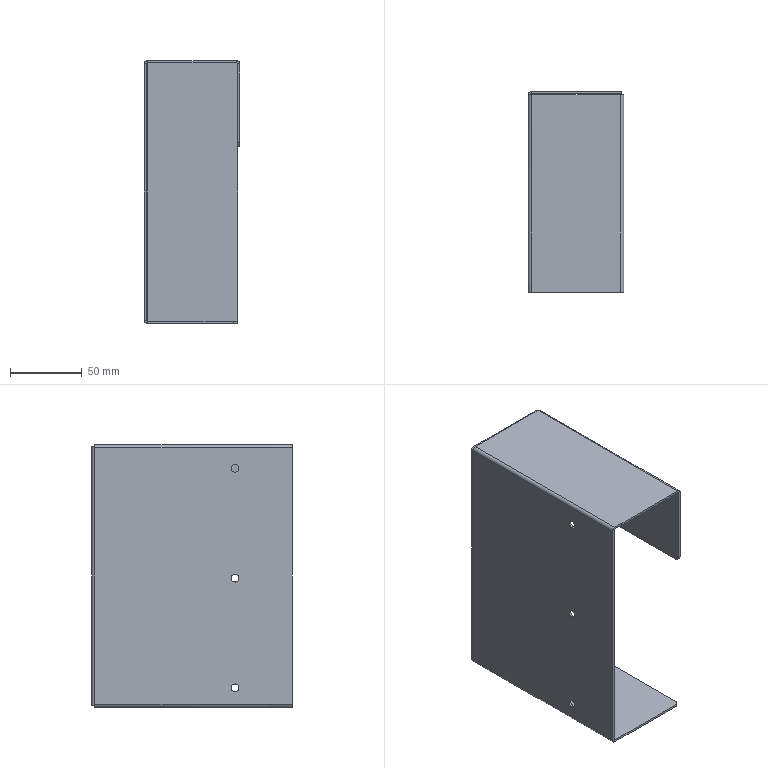Part | SolidWorks | features EdgeFlange 2, Fillet 1, FlatPattern 1, HoleWzd 1, SMBaseFlange 1, SheetMetal 1 | 1 solid | 48 faces | box 66.5 x 140 x 183 mm | volume 93527 mm3 | plane 32 | cylinder 16 | commonest cylinder face diameters 5.5 x6 1.473 x4 4.473 x4 6 x2
STEP:
#1=CARTESIAN_POINT('',(1.5,40.,9.25));
#2=VERTEX_POINT('',#1);
#3=CARTESIAN_POINT('',(1.5,40.,14.75));
#4=VERTEX_POINT('',#3);
#5=CARTESIAN_POINT('',(1.5,40.,12.));
#6=DIRECTION('',(-1.,0.,0.));
#7=DIRECTION('',(0.,0.,1.));
#8=AXIS2_PLACEMENT_3D('',#5,#6,#7);
#9=CIRCLE('',#8,2.75);
#10=EDGE_CURVE('',#2,#4,#9,.T.);
#11=ORIENTED_EDGE('',*,*,#10,.F.);
#12=CARTESIAN_POINT('',(0.,40.,9.25));
#13=VERTEX_POINT('',#12);
#14=CARTESIAN_POINT('',(0.,40.,9.25));
#15=DIRECTION('',(-1.,0.,0.));
#16=VECTOR('',#15,1000.);
#17=LINE('',#14,#16);
#18=EDGE_CURVE('',#2,#13,#17,.T.);
#19=ORIENTED_EDGE('',*,*,#18,.T.);
#20=CARTESIAN_POINT('',(0.,40.,14.75));
#21=VERTEX_POINT('',#20);
#22=CARTESIAN_POINT('',(0.,40.,12.));
#23=DIRECTION('',(-1.,0.,0.));
#24=DIRECTION('',(0.,0.,1.));
#25=AXIS2_PLACEMENT_3D('',#22,#23,#24);
#26=CIRCLE('',#25,2.75);
#27=EDGE_CURVE('',#13,#21,#26,.T.);
#28=ORIENTED_EDGE('',*,*,#27,.T.);
#29=CARTESIAN_POINT('',(0.,40.,14.75));
#30=DIRECTION('',(-1.,0.,0.));
#31=VECTOR('',#30,1000.);
#32=LINE('',#29,#31);
#33=EDGE_CURVE('',#4,#21,#32,.T.);
#34=ORIENTED_EDGE('',*,*,#33,.F.);
#35=EDGE_LOOP('',(#11,#19,#28,#34));
#36=FACE_OUTER_BOUND('',#35,.T.);
#37=CARTESIAN_POINT('',(0.,40.,12.));
#38=DIRECTION('',(-1.,0.,0.));
#39=DIRECTION('',(0.,0.,1.));
#40=AXIS2_PLACEMENT_3D('',#37,#38,#39);
#41=CYLINDRICAL_SURFACE('',#40,2.75);
#42=ADVANCED_FACE('',(#36),#41,.F.);
#43=CARTESIAN_POINT('',(1.5,40.,85.75));
#44=VERTEX_POINT('',#43);
#45=CARTESIAN_POINT('',(1.5,40.,91.25));
#46=VERTEX_POINT('',#45);
#47=CARTESIAN_POINT('',(1.5,40.,88.5));
#48=DIRECTION('',(-1.,0.,0.));
#49=DIRECTION('',(0.,0.,1.));
#50=AXIS2_PLACEMENT_3D('',#47,#48,#49);
#51=CIRCLE('',#50,2.75);
#52=EDGE_CURVE('',#44,#46,#51,.T.);
#53=ORIENTED_EDGE('',*,*,#52,.F.);
#54=CARTESIAN_POINT('',(0.,40.,85.75));
#55=VERTEX_POINT('',#54);
#56=CARTESIAN_POINT('',(0.,40.,85.75));
#57=DIRECTION('',(-1.,0.,0.));
#58=VECTOR('',#57,1000.);
#59=LINE('',#56,#58);
#60=EDGE_CURVE('',#44,#55,#59,.T.);
#61=ORIENTED_EDGE('',*,*,#60,.T.);
#62=CARTESIAN_POINT('',(0.,40.,91.25));
#63=VERTEX_POINT('',#62);
#64=CARTESIAN_POINT('',(0.,40.,88.5));
#65=DIRECTION('',(-1.,0.,0.));
#66=DIRECTION('',(0.,0.,1.));
#67=AXIS2_PLACEMENT_3D('',#64,#65,#66);
#68=CIRCLE('',#67,2.75);
#69=EDGE_CURVE('',#55,#63,#68,.T.);
#70=ORIENTED_EDGE('',*,*,#69,.T.);
#71=CARTESIAN_POINT('',(0.,40.,91.25));
#72=DIRECTION('',(-1.,0.,0.));
#73=VECTOR('',#72,1000.);
#74=LINE('',#71,#73);
#75=EDGE_CURVE('',#46,#63,#74,.T.);
#76=ORIENTED_EDGE('',*,*,#75,.F.);
#77=EDGE_LOOP('',(#53,#61,#70,#76));
#78=FACE_OUTER_BOUND('',#77,.T.);
#79=CARTESIAN_POINT('',(0.,40.,88.5));
#80=DIRECTION('',(-1.,0.,0.));
#81=DIRECTION('',(0.,0.,1.));
#82=AXIS2_PLACEMENT_3D('',#79,#80,#81);
#83=CYLINDRICAL_SURFACE('',#82,2.75);
#84=ADVANCED_FACE('',(#78),#83,.F.);
#85=CARTESIAN_POINT('',(1.5,40.,162.25));
#86=VERTEX_POINT('',#85);
#87=CARTESIAN_POINT('',(1.5,40.,167.75));
#88=VERTEX_POINT('',#87);
#89=CARTESIAN_POINT('',(1.5,40.,165.));
#90=DIRECTION('',(-1.,0.,0.));
#91=DIRECTION('',(0.,0.,1.));
#92=AXIS2_PLACEMENT_3D('',#89,#90,#91);
#93=CIRCLE('',#92,2.75);
#94=EDGE_CURVE('',#86,#88,#93,.T.);
#95=ORIENTED_EDGE('',*,*,#94,.F.);
#96=CARTESIAN_POINT('',(0.,40.,162.25));
#97=VERTEX_POINT('',#96);
#98=CARTESIAN_POINT('',(0.,40.,162.25));
#99=DIRECTION('',(-1.,0.,0.));
#100=VECTOR('',#99,1000.);
#101=LINE('',#98,#100);
#102=EDGE_CURVE('',#86,#97,#101,.T.);
#103=ORIENTED_EDGE('',*,*,#102,.T.);
#104=CARTESIAN_POINT('',(0.,40.,167.75));
#105=VERTEX_POINT('',#104);
#106=CARTESIAN_POINT('',(0.,40.,165.));
#107=DIRECTION('',(-1.,0.,0.));
#108=DIRECTION('',(0.,0.,1.));
#109=AXIS2_PLACEMENT_3D('',#106,#107,#108);
#110=CIRCLE('',#109,2.75);
#111=EDGE_CURVE('',#97,#105,#110,.T.);
#112=ORIENTED_EDGE('',*,*,#111,.T.);
#113=CARTESIAN_POINT('',(0.,40.,167.75));
#114=DIRECTION('',(-1.,0.,0.));
#115=VECTOR('',#114,1000.);
#116=LINE('',#113,#115);
#117=EDGE_CURVE('',#88,#105,#116,.T.);
#118=ORIENTED_EDGE('',*,*,#117,.F.);
#119=EDGE_LOOP('',(#95,#103,#112,#118));
#120=FACE_OUTER_BOUND('',#119,.T.);
#121=CARTESIAN_POINT('',(0.,40.,165.));
#122=DIRECTION('',(-1.,0.,0.));
#123=DIRECTION('',(0.,0.,1.));
#124=AXIS2_PLACEMENT_3D('',#121,#122,#123);
#125=CYLINDRICAL_SURFACE('',#124,2.75);
#126=ADVANCED_FACE('',(#120),#125,.F.);
#127=CARTESIAN_POINT('',(64.263,0.,180.));
#128=VERTEX_POINT('',#127);
#129=CARTESIAN_POINT('',(64.263,0.,181.5));
#130=VERTEX_POINT('',#129);
#131=CARTESIAN_POINT('',(64.263,0.,180.));
#132=DIRECTION('',(0.,0.,1.));
#133=VECTOR('',#132,1000.);
#134=LINE('',#131,#133);
#135=EDGE_CURVE('',#128,#130,#134,.T.);
#136=ORIENTED_EDGE('',*,*,#135,.T.);
#137=CARTESIAN_POINT('',(2.237,0.,181.5));
#138=VERTEX_POINT('',#137);
#139=CARTESIAN_POINT('',(65.,0.,181.5));
#140=DIRECTION('',(1.,0.,0.));
#141=VECTOR('',#140,1000.);
#142=LINE('',#139,#141);
#143=EDGE_CURVE('',#138,#130,#142,.T.);
#144=ORIENTED_EDGE('',*,*,#143,.F.);
#145=CARTESIAN_POINT('',(2.237,0.,180.));
#146=VERTEX_POINT('',#145);
#147=CARTESIAN_POINT('',(2.237,0.,180.));
#148=DIRECTION('',(0.,0.,1.));
#149=VECTOR('',#148,1000.);
#150=LINE('',#147,#149);
#151=EDGE_CURVE('',#146,#138,#150,.T.);
#152=ORIENTED_EDGE('',*,*,#151,.F.);
#153=CARTESIAN_POINT('',(65.,0.,180.));
#154=DIRECTION('',(1.,0.,0.));
#155=VECTOR('',#154,1000.);
#156=LINE('',#153,#155);
#157=EDGE_CURVE('',#146,#128,#156,.T.);
#158=ORIENTED_EDGE('',*,*,#157,.T.);
#159=EDGE_LOOP('',(#136,#144,#152,#158));
#160=FACE_OUTER_BOUND('',#159,.T.);
#161=CARTESIAN_POINT('',(65.,0.,181.5));
#162=DIRECTION('',(0.,1.,0.));
#163=DIRECTION('',(0.,0.,1.));
#164=AXIS2_PLACEMENT_3D('',#161,#162,#163);
#165=PLANE('',#164);
#166=ADVANCED_FACE('',(#160),#165,.F.);
#167=CARTESIAN_POINT('',(64.263,137.763,180.));
#168=VERTEX_POINT('',#167);
#169=CARTESIAN_POINT('',(64.263,137.763,181.5));
#170=VERTEX_POINT('',#169);
#171=CARTESIAN_POINT('',(64.263,137.763,180.));
#172=DIRECTION('',(0.,0.,1.));
#173=VECTOR('',#172,1000.);
#174=LINE('',#171,#173);
#175=EDGE_CURVE('',#168,#170,#174,.T.);
#176=ORIENTED_EDGE('',*,*,#175,.F.);
#177=CARTESIAN_POINT('',(2.237,137.763,180.));
#178=VERTEX_POINT('',#177);
#179=CARTESIAN_POINT('',(1.5,137.763,180.));
#180=DIRECTION('',(-1.,0.,0.));
#181=VECTOR('',#180,1000.);
#182=LINE('',#179,#181);
#183=EDGE_CURVE('',#168,#178,#182,.T.);
#184=ORIENTED_EDGE('',*,*,#183,.T.);
#185=CARTESIAN_POINT('',(2.237,137.763,181.5));
#186=VERTEX_POINT('',#185);
#187=CARTESIAN_POINT('',(2.237,137.763,180.));
#188=DIRECTION('',(0.,0.,1.));
#189=VECTOR('',#188,1000.);
#190=LINE('',#187,#189);
#191=EDGE_CURVE('',#178,#186,#190,.T.);
#192=ORIENTED_EDGE('',*,*,#191,.T.);
#193=CARTESIAN_POINT('',(1.5,137.763,181.5));
#194=DIRECTION('',(-1.,0.,0.));
#195=VECTOR('',#194,1000.);
#196=LINE('',#193,#195);
#197=EDGE_CURVE('',#170,#186,#196,.T.);
#198=ORIENTED_EDGE('',*,*,#197,.F.);
#199=EDGE_LOOP('',(#176,#184,#192,#198));
#200=FACE_OUTER_BOUND('',#199,.T.);
#201=CARTESIAN_POINT('',(1.5,137.763,181.5));
#202=DIRECTION('',(0.,-1.,0.));
#203=DIRECTION('',(0.,0.,-1.));
#204=AXIS2_PLACEMENT_3D('',#201,#202,#203);
#205=PLANE('',#204);
#206=ADVANCED_FACE('',(#200),#205,.F.);
#207=CARTESIAN_POINT('',(64.263,0.,181.5));
#208=DIRECTION('',(0.,1.,0.));
#209=VECTOR('',#208,1000.);
#210=LINE('',#207,#209);
#211=EDGE_CURVE('',#130,#170,#210,.T.);
#212=ORIENTED_EDGE('',*,*,#211,.T.);
#213=ORIENTED_EDGE('',*,*,#197,.T.);
#214=CARTESIAN_POINT('',(2.237,0.,181.5));
#215=DIRECTION('',(0.,1.,0.));
#216=VECTOR('',#215,1000.);
#217=LINE('',#214,#216);
#218=EDGE_CURVE('',#138,#186,#217,.T.);
#219=ORIENTED_EDGE('',*,*,#218,.F.);
#220=ORIENTED_EDGE('',*,*,#143,.T.);
#221=EDGE_LOOP('',(#212,#213,#219,#220));
#222=FACE_OUTER_BOUND('',#221,.T.);
#223=CARTESIAN_POINT('',(0.,0.,181.5));
#224=DIRECTION('',(0.,0.,-1.));
#225=DIRECTION('',(-1.,0.,0.));
#226=AXIS2_PLACEMENT_3D('',#223,#224,#225);
#227=PLANE('',#226);
#228=ADVANCED_FACE('',(#222),#227,.F.);
#229=ORIENTED_EDGE('',*,*,#183,.F.);
#230=CARTESIAN_POINT('',(64.263,0.,180.));
#231=DIRECTION('',(0.,1.,0.));
#232=VECTOR('',#231,1000.);
#233=LINE('',#230,#232);
#234=EDGE_CURVE('',#128,#168,#233,.T.);
#235=ORIENTED_EDGE('',*,*,#234,.F.);
#236=ORIENTED_EDGE('',*,*,#157,.F.);
#237=CARTESIAN_POINT('',(2.237,137.763,180.));
#238=DIRECTION('',(0.,-1.,0.));
#239=VECTOR('',#238,1000.);
#240=LINE('',#237,#239);
#241=EDGE_CURVE('',#178,#146,#240,.T.);
#242=ORIENTED_EDGE('',*,*,#241,.F.);
#243=EDGE_LOOP('',(#229,#235,#236,#242));
#244=FACE_OUTER_BOUND('',#243,.T.);
#245=CARTESIAN_POINT('',(0.,0.,180.));
#246=DIRECTION('',(0.,0.,-1.));
#247=DIRECTION('',(-1.,0.,0.));
#248=AXIS2_PLACEMENT_3D('',#245,#246,#247);
#249=PLANE('',#248);
#250=ADVANCED_FACE('',(#244),#249,.T.);
#251=CARTESIAN_POINT('',(0.,137.763,180.));
#252=VERTEX_POINT('',#251);
#253=CARTESIAN_POINT('',(0.,137.763,179.263));
#254=VERTEX_POINT('',#253);
#255=CARTESIAN_POINT('',(0.,137.763,180.));
#256=DIRECTION('',(0.,0.,-1.));
#257=VECTOR('',#256,1000.);
#258=LINE('',#255,#257);
#259=EDGE_CURVE('',#252,#254,#258,.T.);
#260=ORIENTED_EDGE('',*,*,#259,.T.);
#261=CARTESIAN_POINT('',(0.1248,137.763,180.));
#262=VERTEX_POINT('',#261);
#263=CARTESIAN_POINT('',(2.237,137.763,179.263));
#264=DIRECTION('',(0.,1.,0.));
#265=DIRECTION('',(0.,0.,-1.));
#266=AXIS2_PLACEMENT_3D('',#263,#264,#265);
#267=CIRCLE('',#266,2.237);
#268=EDGE_CURVE('',#254,#262,#267,.T.);
#269=ORIENTED_EDGE('',*,*,#268,.T.);
#270=CARTESIAN_POINT('',(1.5,137.763,180.));
#271=DIRECTION('',(-1.,0.,0.));
#272=VECTOR('',#271,1000.);
#273=LINE('',#270,#272);
#274=EDGE_CURVE('',#262,#252,#273,.T.);
#275=ORIENTED_EDGE('',*,*,#274,.T.);
#276=EDGE_LOOP('',(#260,#269,#275));
#277=FACE_OUTER_BOUND('',#276,.T.);
#278=CARTESIAN_POINT('',(1.5,137.763,179.263));
#279=DIRECTION('',(0.,-1.,0.));
#280=DIRECTION('',(0.,0.,-1.));
#281=AXIS2_PLACEMENT_3D('',#278,#279,#280);
#282=PLANE('',#281);
#283=ADVANCED_FACE('',(#277),#282,.T.);
#284=CARTESIAN_POINT('',(0.,137.763,0.));
#285=VERTEX_POINT('',#284);
#286=CARTESIAN_POINT('',(0.1248,137.763,0.));
#287=VERTEX_POINT('',#286);
#288=CARTESIAN_POINT('',(0.,137.763,0.));
#289=DIRECTION('',(1.,0.,0.));
#290=VECTOR('',#289,1000.);
#291=LINE('',#288,#290);
#292=EDGE_CURVE('',#285,#287,#291,.T.);
#293=ORIENTED_EDGE('',*,*,#292,.T.);
#294=CARTESIAN_POINT('',(0.,137.763,0.7366));
#295=VERTEX_POINT('',#294);
#296=CARTESIAN_POINT('',(2.237,137.763,0.7366));
#297=DIRECTION('',(0.,1.,0.));
#298=DIRECTION('',(0.,0.,1.));
#299=AXIS2_PLACEMENT_3D('',#296,#297,#298);
#300=CIRCLE('',#299,2.237);
#301=EDGE_CURVE('',#287,#295,#300,.T.);
#302=ORIENTED_EDGE('',*,*,#301,.T.);
#303=CARTESIAN_POINT('',(0.,137.763,180.));
#304=DIRECTION('',(0.,0.,1.));
#305=VECTOR('',#304,1000.);
#306=LINE('',#303,#305);
#307=EDGE_CURVE('',#285,#295,#306,.T.);
#308=ORIENTED_EDGE('',*,*,#307,.F.);
#309=EDGE_LOOP('',(#293,#302,#308));
#310=FACE_OUTER_BOUND('',#309,.T.);
#311=CARTESIAN_POINT('',(1.5,137.763,0.));
#312=DIRECTION('',(0.,-1.,0.));
#313=DIRECTION('',(0.,0.,-1.));
#314=AXIS2_PLACEMENT_3D('',#311,#312,#313);
#315=PLANE('',#314);
#316=ADVANCED_FACE('',(#310),#315,.T.);
#317=CARTESIAN_POINT('',(0.,40.,12.));
#318=DIRECTION('',(-1.,0.,0.));
#319=DIRECTION('',(0.,0.,1.));
#320=AXIS2_PLACEMENT_3D('',#317,#318,#319);
#321=CIRCLE('',#320,2.75);
#322=EDGE_CURVE('',#21,#13,#321,.T.);
#323=ORIENTED_EDGE('',*,*,#322,.F.);
#324=ORIENTED_EDGE('',*,*,#27,.F.);
#325=EDGE_LOOP('',(#323,#324));
#326=FACE_BOUND('',#325,.T.);
#327=CARTESIAN_POINT('',(0.,40.,88.5));
#328=DIRECTION('',(-1.,0.,0.));
#329=DIRECTION('',(0.,0.,1.));
#330=AXIS2_PLACEMENT_3D('',#327,#328,#329);
#331=CIRCLE('',#330,2.75);
#332=EDGE_CURVE('',#63,#55,#331,.T.);
#333=ORIENTED_EDGE('',*,*,#332,.F.);
#334=ORIENTED_EDGE('',*,*,#69,.F.);
#335=EDGE_LOOP('',(#333,#334));
#336=FACE_BOUND('',#335,.T.);
#337=CARTESIAN_POINT('',(0.,40.,165.));
#338=DIRECTION('',(-1.,0.,0.));
#339=DIRECTION('',(0.,0.,1.));
#340=AXIS2_PLACEMENT_3D('',#337,#338,#339);
#341=CIRCLE('',#340,2.75);
#342=EDGE_CURVE('',#105,#97,#341,.T.);
#343=ORIENTED_EDGE('',*,*,#342,.F.);
#344=ORIENTED_EDGE('',*,*,#111,.F.);
#345=EDGE_LOOP('',(#343,#344));
#346=FACE_BOUND('',#345,.T.);
#347=CARTESIAN_POINT('',(0.,0.,179.263));
#348=VERTEX_POINT('',#347);
#349=CARTESIAN_POINT('',(0.,0.,0.7366));
#350=VERTEX_POINT('',#349);
#351=CARTESIAN_POINT('',(0.,0.,180.));
#352=DIRECTION('',(0.,0.,-1.));
#353=VECTOR('',#352,1000.);
#354=LINE('',#351,#353);
#355=EDGE_CURVE('',#348,#350,#354,.T.);
#356=ORIENTED_EDGE('',*,*,#355,.F.);
#357=CARTESIAN_POINT('',(0.,0.,179.263));
#358=DIRECTION('',(0.,1.,0.));
#359=VECTOR('',#358,1000.);
#360=LINE('',#357,#359);
#361=EDGE_CURVE('',#348,#254,#360,.T.);
#362=ORIENTED_EDGE('',*,*,#361,.T.);
#363=CARTESIAN_POINT('',(0.,137.763,180.));
#364=DIRECTION('',(0.,0.,-1.));
#365=VECTOR('',#364,1000.);
#366=LINE('',#363,#365);
#367=EDGE_CURVE('',#254,#295,#366,.T.);
#368=ORIENTED_EDGE('',*,*,#367,.T.);
#369=CARTESIAN_POINT('',(0.,137.763,0.7366));
#370=DIRECTION('',(0.,-1.,0.));
#371=VECTOR('',#370,1000.);
#372=LINE('',#369,#371);
#373=EDGE_CURVE('',#295,#350,#372,.T.);
#374=ORIENTED_EDGE('',*,*,#373,.T.);
#375=EDGE_LOOP('',(#356,#362,#368,#374));
#376=FACE_OUTER_BOUND('',#375,.T.);
#377=CARTESIAN_POINT('',(0.,0.,180.));
#378=DIRECTION('',(-1.,0.,0.));
#379=DIRECTION('',(0.,0.,1.));
#380=AXIS2_PLACEMENT_3D('',#377,#378,#379);
#381=PLANE('',#380);
#382=ADVANCED_FACE('',(#326,#336,#346,#376),#381,.T.);
#383=CARTESIAN_POINT('',(1.5,40.,12.));
#384=DIRECTION('',(-1.,0.,0.));
#385=DIRECTION('',(0.,0.,1.));
#386=AXIS2_PLACEMENT_3D('',#383,#384,#385);
#387=CIRCLE('',#386,2.75);
#388=EDGE_CURVE('',#4,#2,#387,.T.);
#389=ORIENTED_EDGE('',*,*,#388,.T.);
#390=ORIENTED_EDGE('',*,*,#10,.T.);
#391=EDGE_LOOP('',(#389,#390));
#392=FACE_BOUND('',#391,.T.);
#393=CARTESIAN_POINT('',(1.5,40.,88.5));
#394=DIRECTION('',(-1.,0.,0.));
#395=DIRECTION('',(0.,0.,1.));
#396=AXIS2_PLACEMENT_3D('',#393,#394,#395);
#397=CIRCLE('',#396,2.75);
#398=EDGE_CURVE('',#46,#44,#397,.T.);
#399=ORIENTED_EDGE('',*,*,#398,.T.);
#400=ORIENTED_EDGE('',*,*,#52,.T.);
#401=EDGE_LOOP('',(#399,#400));
#402=FACE_BOUND('',#401,.T.);
#403=CARTESIAN_POINT('',(1.5,40.,165.));
#404=DIRECTION('',(-1.,0.,0.));
#405=DIRECTION('',(0.,0.,1.));
#406=AXIS2_PLACEMENT_3D('',#403,#404,#405);
#407=CIRCLE('',#406,2.75);
#408=EDGE_CURVE('',#88,#86,#407,.T.);
#409=ORIENTED_EDGE('',*,*,#408,.T.);
#410=ORIENTED_EDGE('',*,*,#94,.T.);
#411=EDGE_LOOP('',(#409,#410));
#412=FACE_BOUND('',#411,.T.);
#413=CARTESIAN_POINT('',(1.5,0.,179.263));
#414=VERTEX_POINT('',#413);
#415=CARTESIAN_POINT('',(1.5,137.763,179.263));
#416=VERTEX_POINT('',#415);
#417=CARTESIAN_POINT('',(1.5,0.,179.263));
#418=DIRECTION('',(0.,1.,0.));
#419=VECTOR('',#418,1000.);
#420=LINE('',#417,#419);
#421=EDGE_CURVE('',#414,#416,#420,.T.);
#422=ORIENTED_EDGE('',*,*,#421,.F.);
#423=CARTESIAN_POINT('',(1.5,0.,0.7366));
#424=VERTEX_POINT('',#423);
#425=CARTESIAN_POINT('',(1.5,0.,180.));
#426=DIRECTION('',(0.,0.,-1.));
#427=VECTOR('',#426,1000.);
#428=LINE('',#425,#427);
#429=EDGE_CURVE('',#414,#424,#428,.T.);
#430=ORIENTED_EDGE('',*,*,#429,.T.);
#431=CARTESIAN_POINT('',(1.5,137.763,0.7366));
#432=VERTEX_POINT('',#431);
#433=CARTESIAN_POINT('',(1.5,137.763,0.7366));
#434=DIRECTION('',(0.,-1.,0.));
#435=VECTOR('',#434,1000.);
#436=LINE('',#433,#435);
#437=EDGE_CURVE('',#432,#424,#436,.T.);
#438=ORIENTED_EDGE('',*,*,#437,.F.);
#439=CARTESIAN_POINT('',(1.5,137.763,180.));
#440=DIRECTION('',(0.,0.,-1.));
#441=VECTOR('',#440,1000.);
#442=LINE('',#439,#441);
#443=EDGE_CURVE('',#416,#432,#442,.T.);
#444=ORIENTED_EDGE('',*,*,#443,.F.);
#445=EDGE_LOOP('',(#422,#430,#438,#444));
#446=FACE_OUTER_BOUND('',#445,.T.);
#447=CARTESIAN_POINT('',(1.5,0.,180.));
#448=DIRECTION('',(-1.,0.,0.));
#449=DIRECTION('',(0.,0.,1.));
#450=AXIS2_PLACEMENT_3D('',#447,#448,#449);
#451=PLANE('',#450);
#452=ADVANCED_FACE('',(#392,#402,#412,#446),#451,.F.);
#453=ORIENTED_EDGE('',*,*,#429,.F.);
#454=CARTESIAN_POINT('',(1.5,0.,179.263));
#455=DIRECTION('',(-1.,0.,0.));
#456=VECTOR('',#455,1000.);
#457=LINE('',#454,#456);
#458=EDGE_CURVE('',#414,#348,#457,.T.);
#459=ORIENTED_EDGE('',*,*,#458,.T.);
#460=ORIENTED_EDGE('',*,*,#355,.T.);
#461=CARTESIAN_POINT('',(1.5,0.,0.7366));
#462=DIRECTION('',(-1.,0.,0.));
#463=VECTOR('',#462,1000.);
#464=LINE('',#461,#463);
#465=EDGE_CURVE('',#424,#350,#464,.T.);
#466=ORIENTED_EDGE('',*,*,#465,.F.);
#467=EDGE_LOOP('',(#453,#459,#460,#466));
#468=FACE_OUTER_BOUND('',#467,.T.);
#469=CARTESIAN_POINT('',(1.5,0.,180.));
#470=DIRECTION('',(0.,-1.,0.));
#471=DIRECTION('',(0.,0.,-1.));
#472=AXIS2_PLACEMENT_3D('',#469,#470,#471);
#473=PLANE('',#472);
#474=ADVANCED_FACE('',(#468),#473,.T.);
#475=CARTESIAN_POINT('',(2.237,140.,180.));
#476=VERTEX_POINT('',#475);
#477=CARTESIAN_POINT('',(2.237,138.5,180.));
#478=VERTEX_POINT('',#477);
#479=CARTESIAN_POINT('',(2.237,140.,180.));
#480=DIRECTION('',(0.,-1.,0.));
#481=VECTOR('',#480,1000.);
#482=LINE('',#479,#481);
#483=EDGE_CURVE('',#476,#478,#482,.T.);
#484=ORIENTED_EDGE('',*,*,#483,.F.);
#485=CARTESIAN_POINT('',(2.237,137.763,180.));
#486=DIRECTION('',(0.,0.,-1.));
#487=DIRECTION('',(1.,0.,0.));
#488=AXIS2_PLACEMENT_3D('',#485,#486,#487);
#489=CIRCLE('',#488,2.237);
#490=EDGE_CURVE('',#252,#476,#489,.T.);
#491=ORIENTED_EDGE('',*,*,#490,.F.);
#492=ORIENTED_EDGE('',*,*,#274,.F.);
#493=CARTESIAN_POINT('',(1.5,137.763,180.));
#494=VERTEX_POINT('',#493);
#495=CARTESIAN_POINT('',(1.5,137.763,180.));
#496=DIRECTION('',(-1.,0.,0.));
#497=VECTOR('',#496,1000.);
#498=LINE('',#495,#497);
#499=EDGE_CURVE('',#494,#262,#498,.T.);
#500=ORIENTED_EDGE('',*,*,#499,.F.);
#501=CARTESIAN_POINT('',(2.237,137.763,180.));
#502=DIRECTION('',(0.,0.,-1.));
#503=DIRECTION('',(1.,0.,0.));
#504=AXIS2_PLACEMENT_3D('',#501,#502,#503);
#505=CIRCLE('',#504,0.7366);
#506=EDGE_CURVE('',#494,#478,#505,.T.);
#507=ORIENTED_EDGE('',*,*,#506,.T.);
#508=EDGE_LOOP('',(#484,#491,#492,#500,#507));
#509=FACE_OUTER_BOUND('',#508,.T.);
#510=CARTESIAN_POINT('',(2.237,140.,180.));
#511=DIRECTION('',(0.,0.,1.));
#512=DIRECTION('',(1.,0.,0.));
#513=AXIS2_PLACEMENT_3D('',#510,#511,#512);
#514=PLANE('',#513);
#515=ADVANCED_FACE('',(#509),#514,.T.);
#516=CARTESIAN_POINT('',(65.,140.,180.));
#517=VERTEX_POINT('',#516);
#518=CARTESIAN_POINT('',(0.,140.,180.));
#519=DIRECTION('',(1.,0.,0.));
#520=VECTOR('',#519,1000.);
#521=LINE('',#518,#520);
#522=EDGE_CURVE('',#476,#517,#521,.T.);
#523=ORIENTED_EDGE('',*,*,#522,.F.);
#524=ORIENTED_EDGE('',*,*,#483,.T.);
#525=CARTESIAN_POINT('',(65.,138.5,180.));
#526=VERTEX_POINT('',#525);
#527=CARTESIAN_POINT('',(0.,138.5,180.));
#528=DIRECTION('',(1.,0.,0.));
#529=VECTOR('',#528,1000.);
#530=LINE('',#527,#529);
#531=EDGE_CURVE('',#478,#526,#530,.T.);
#532=ORIENTED_EDGE('',*,*,#531,.T.);
#533=CARTESIAN_POINT('',(65.,140.,180.));
#534=DIRECTION('',(0.,-1.,0.));
#535=VECTOR('',#534,1000.);
#536=LINE('',#533,#535);
#537=EDGE_CURVE('',#517,#526,#536,.T.);
#538=ORIENTED_EDGE('',*,*,#537,.F.);
#539=EDGE_LOOP('',(#523,#524,#532,#538));
#540=FACE_OUTER_BOUND('',#539,.T.);
#541=CARTESIAN_POINT('',(1.5,137.763,180.));
#542=DIRECTION('',(0.,0.,1.));
#543=DIRECTION('',(1.,0.,0.));
#544=AXIS2_PLACEMENT_3D('',#541,#542,#543);
#545=PLANE('',#544);
#546=ADVANCED_FACE('',(#540),#545,.T.);
#547=ORIENTED_EDGE('',*,*,#292,.F.);
#548=CARTESIAN_POINT('',(2.237,140.,0.));
#549=VERTEX_POINT('',#548);
#550=CARTESIAN_POINT('',(2.237,137.763,0.));
#551=DIRECTION('',(0.,0.,-1.));
#552=DIRECTION('',(1.,0.,0.));
#553=AXIS2_PLACEMENT_3D('',#550,#551,#552);
#554=CIRCLE('',#553,2.237);
#555=EDGE_CURVE('',#285,#549,#554,.T.);
#556=ORIENTED_EDGE('',*,*,#555,.T.);
#557=CARTESIAN_POINT('',(2.237,138.5,0.));
#558=VERTEX_POINT('',#557);
#559=CARTESIAN_POINT('',(2.237,138.5,0.));
#560=DIRECTION('',(0.,1.,0.));
#561=VECTOR('',#560,1000.);
#562=LINE('',#559,#561);
#563=EDGE_CURVE('',#558,#549,#562,.T.);
#564=ORIENTED_EDGE('',*,*,#563,.F.);
#565=CARTESIAN_POINT('',(1.5,137.763,0.));
#566=VERTEX_POINT('',#565);
#567=CARTESIAN_POINT('',(2.237,137.763,0.));
#568=DIRECTION('',(0.,0.,-1.));
#569=DIRECTION('',(1.,0.,0.));
#570=AXIS2_PLACEMENT_3D('',#567,#568,#569);
#571=CIRCLE('',#570,0.7366);
#572=EDGE_CURVE('',#566,#558,#571,.T.);
#573=ORIENTED_EDGE('',*,*,#572,.F.);
#574=CARTESIAN_POINT('',(0.,137.763,0.));
#575=DIRECTION('',(1.,0.,0.));
#576=VECTOR('',#575,1000.);
#577=LINE('',#574,#576);
#578=EDGE_CURVE('',#287,#566,#577,.T.);
#579=ORIENTED_EDGE('',*,*,#578,.F.);
#580=EDGE_LOOP('',(#547,#556,#564,#573,#579));
#581=FACE_OUTER_BOUND('',#580,.T.);
#582=CARTESIAN_POINT('',(0.,137.763,0.));
#583=DIRECTION('',(0.,0.,-1.));
#584=DIRECTION('',(-1.,0.,0.));
#585=AXIS2_PLACEMENT_3D('',#582,#583,#584);
#586=PLANE('',#585);
#587=ADVANCED_FACE('',(#581),#586,.T.);
#588=CARTESIAN_POINT('',(65.,138.5,0.));
#589=VERTEX_POINT('',#588);
#590=CARTESIAN_POINT('',(0.,138.5,0.));
#591=DIRECTION('',(1.,0.,0.));
#592=VECTOR('',#591,1000.);
#593=LINE('',#590,#592);
#594=EDGE_CURVE('',#558,#589,#593,.T.);
#595=ORIENTED_EDGE('',*,*,#594,.T.);
#596=CARTESIAN_POINT('',(65.,138.5,180.));
#597=DIRECTION('',(0.,0.,-1.));
#598=VECTOR('',#597,1000.);
#599=LINE('',#596,#598);
#600=EDGE_CURVE('',#526,#589,#599,.T.);
#601=ORIENTED_EDGE('',*,*,#600,.F.);
#602=ORIENTED_EDGE('',*,*,#531,.F.);
#603=CARTESIAN_POINT('',(2.237,138.5,180.));
#604=DIRECTION('',(0.,0.,-1.));
#605=VECTOR('',#604,1000.);
#606=LINE('',#603,#605);
#607=EDGE_CURVE('',#478,#558,#606,.T.);
#608=ORIENTED_EDGE('',*,*,#607,.T.);
#609=EDGE_LOOP('',(#595,#601,#602,#608));
#610=FACE_OUTER_BOUND('',#609,.T.);
#611=CARTESIAN_POINT('',(0.,138.5,180.));
#612=DIRECTION('',(0.,1.,0.));
#613=DIRECTION('',(0.,0.,1.));
#614=AXIS2_PLACEMENT_3D('',#611,#612,#613);
#615=PLANE('',#614);
#616=ADVANCED_FACE('',(#610),#615,.F.);
#617=CARTESIAN_POINT('',(65.,140.,0.));
#618=VERTEX_POINT('',#617);
#619=CARTESIAN_POINT('',(65.,140.,0.));
#620=DIRECTION('',(0.,-1.,0.));
#621=VECTOR('',#620,1000.);
#622=LINE('',#619,#621);
#623=EDGE_CURVE('',#618,#589,#622,.T.);
#624=ORIENTED_EDGE('',*,*,#623,.F.);
#625=CARTESIAN_POINT('',(65.,140.,180.));
#626=DIRECTION('',(0.,0.,-1.));
#627=VECTOR('',#626,1000.);
#628=LINE('',#625,#627);
#629=EDGE_CURVE('',#517,#618,#628,.T.);
#630=ORIENTED_EDGE('',*,*,#629,.F.);
#631=ORIENTED_EDGE('',*,*,#537,.T.);
#632=ORIENTED_EDGE('',*,*,#600,.T.);
#633=EDGE_LOOP('',(#624,#630,#631,#632));
#634=FACE_OUTER_BOUND('',#633,.T.);
#635=CARTESIAN_POINT('',(65.,140.,180.));
#636=DIRECTION('',(1.,0.,0.));
#637=DIRECTION('',(0.,0.,-1.));
#638=AXIS2_PLACEMENT_3D('',#635,#636,#637);
#639=PLANE('',#638);
#640=ADVANCED_FACE('',(#634),#639,.T.);
#641=CARTESIAN_POINT('',(0.,140.,0.));
#642=DIRECTION('',(1.,0.,0.));
#643=VECTOR('',#642,1000.);
#644=LINE('',#641,#643);
#645=EDGE_CURVE('',#549,#618,#644,.T.);
#646=ORIENTED_EDGE('',*,*,#645,.F.);
#647=CARTESIAN_POINT('',(2.237,140.,180.));
#648=DIRECTION('',(0.,0.,-1.));
#649=VECTOR('',#648,1000.);
#650=LINE('',#647,#649);
#651=EDGE_CURVE('',#476,#549,#650,.T.);
#652=ORIENTED_EDGE('',*,*,#651,.F.);
#653=ORIENTED_EDGE('',*,*,#522,.T.);
#654=ORIENTED_EDGE('',*,*,#629,.T.);
#655=EDGE_LOOP('',(#646,#652,#653,#654));
#656=FACE_OUTER_BOUND('',#655,.T.);
#657=CARTESIAN_POINT('',(0.,140.,180.));
#658=DIRECTION('',(0.,1.,0.));
#659=DIRECTION('',(0.,0.,1.));
#660=AXIS2_PLACEMENT_3D('',#657,#658,#659);
#661=PLANE('',#660);
#662=ADVANCED_FACE('',(#656),#661,.T.);
#663=ORIENTED_EDGE('',*,*,#555,.F.);
#664=ORIENTED_EDGE('',*,*,#307,.T.);
#665=ORIENTED_EDGE('',*,*,#367,.F.);
#666=ORIENTED_EDGE('',*,*,#259,.F.);
#667=ORIENTED_EDGE('',*,*,#490,.T.);
#668=ORIENTED_EDGE('',*,*,#651,.T.);
#669=EDGE_LOOP('',(#663,#664,#665,#666,#667,#668));
#670=FACE_OUTER_BOUND('',#669,.T.);
#671=CARTESIAN_POINT('',(2.237,137.763,180.));
#672=DIRECTION('',(0.,0.,-1.));
#673=DIRECTION('',(-1.,0.,0.));
#674=AXIS2_PLACEMENT_3D('',#671,#672,#673);
#675=CYLINDRICAL_SURFACE('',#674,2.237);
#676=ADVANCED_FACE('',(#670),#675,.T.);
#677=ORIENTED_EDGE('',*,*,#572,.T.);
#678=ORIENTED_EDGE('',*,*,#607,.F.);
#679=ORIENTED_EDGE('',*,*,#506,.F.);
#680=CARTESIAN_POINT('',(1.5,137.763,180.));
#681=DIRECTION('',(0.,0.,-1.));
#682=VECTOR('',#681,1000.);
#683=LINE('',#680,#682);
#684=EDGE_CURVE('',#494,#416,#683,.T.);
#685=ORIENTED_EDGE('',*,*,#684,.T.);
#686=ORIENTED_EDGE('',*,*,#443,.T.);
#687=CARTESIAN_POINT('',(1.5,137.763,0.));
#688=DIRECTION('',(0.,0.,1.));
#689=VECTOR('',#688,1000.);
#690=LINE('',#687,#689);
#691=EDGE_CURVE('',#566,#432,#690,.T.);
#692=ORIENTED_EDGE('',*,*,#691,.F.);
#693=EDGE_LOOP('',(#677,#678,#679,#685,#686,#692));
#694=FACE_OUTER_BOUND('',#693,.T.);
#695=CARTESIAN_POINT('',(2.237,137.763,180.));
#696=DIRECTION('',(0.,0.,-1.));
#697=DIRECTION('',(-1.,0.,0.));
#698=AXIS2_PLACEMENT_3D('',#695,#696,#697);
#699=CYLINDRICAL_SURFACE('',#698,0.7366);
#700=ADVANCED_FACE('',(#694),#699,.F.);
#701=ORIENTED_EDGE('',*,*,#594,.F.);
#702=ORIENTED_EDGE('',*,*,#563,.T.);
#703=ORIENTED_EDGE('',*,*,#645,.T.);
#704=ORIENTED_EDGE('',*,*,#623,.T.);
#705=EDGE_LOOP('',(#701,#702,#703,#704));
#706=FACE_OUTER_BOUND('',#705,.T.);
#707=CARTESIAN_POINT('',(2.237,137.763,0.));
#708=DIRECTION('',(0.,0.,1.));
#709=DIRECTION('',(1.,0.,0.));
#710=AXIS2_PLACEMENT_3D('',#707,#708,#709);
#711=PLANE('',#710);
#712=ADVANCED_FACE('',(#706),#711,.F.);
#713=ORIENTED_EDGE('',*,*,#102,.F.);
#714=ORIENTED_EDGE('',*,*,#408,.F.);
#715=ORIENTED_EDGE('',*,*,#117,.T.);
#716=ORIENTED_EDGE('',*,*,#342,.T.);
#717=EDGE_LOOP('',(#713,#714,#715,#716));
#718=FACE_OUTER_BOUND('',#717,.T.);
#719=CARTESIAN_POINT('',(0.,40.,165.));
#720=DIRECTION('',(-1.,0.,0.));
#721=DIRECTION('',(0.,0.,1.));
#722=AXIS2_PLACEMENT_3D('',#719,#720,#721);
#723=CYLINDRICAL_SURFACE('',#722,2.75);
#724=ADVANCED_FACE('',(#718),#723,.F.);
#725=ORIENTED_EDGE('',*,*,#60,.F.);
#726=ORIENTED_EDGE('',*,*,#398,.F.);
#727=ORIENTED_EDGE('',*,*,#75,.T.);
#728=ORIENTED_EDGE('',*,*,#332,.T.);
#729=EDGE_LOOP('',(#725,#726,#727,#728));
#730=FACE_OUTER_BOUND('',#729,.T.);
#731=CARTESIAN_POINT('',(0.,40.,88.5));
#732=DIRECTION('',(-1.,0.,0.));
#733=DIRECTION('',(0.,0.,1.));
#734=AXIS2_PLACEMENT_3D('',#731,#732,#733);
#735=CYLINDRICAL_SURFACE('',#734,2.75);
#736=ADVANCED_FACE('',(#730),#735,.F.);
#737=ORIENTED_EDGE('',*,*,#18,.F.);
#738=ORIENTED_EDGE('',*,*,#388,.F.);
#739=ORIENTED_EDGE('',*,*,#33,.T.);
#740=ORIENTED_EDGE('',*,*,#322,.T.);
#741=EDGE_LOOP('',(#737,#738,#739,#740));
#742=FACE_OUTER_BOUND('',#741,.T.);
#743=CARTESIAN_POINT('',(0.,40.,12.));
#744=DIRECTION('',(-1.,0.,0.));
#745=DIRECTION('',(0.,0.,1.));
#746=AXIS2_PLACEMENT_3D('',#743,#744,#745);
#747=CYLINDRICAL_SURFACE('',#746,2.75);
#748=ADVANCED_FACE('',(#742),#747,.F.);
#749=CARTESIAN_POINT('',(2.237,0.,0.));
#750=VERTEX_POINT('',#749);
#751=CARTESIAN_POINT('',(2.237,0.,-1.5));
#752=VERTEX_POINT('',#751);
#753=CARTESIAN_POINT('',(2.237,0.,0.));
#754=DIRECTION('',(0.,0.,-1.));
#755=VECTOR('',#754,1000.);
#756=LINE('',#753,#755);
#757=EDGE_CURVE('',#750,#752,#756,.T.);
#758=ORIENTED_EDGE('',*,*,#757,.F.);
#759=CARTESIAN_POINT('',(2.237,0.,0.7366));
#760=DIRECTION('',(0.,-1.,0.));
#761=DIRECTION('',(0.,0.,1.));
#762=AXIS2_PLACEMENT_3D('',#759,#760,#761);
#763=CIRCLE('',#762,0.7366);
#764=EDGE_CURVE('',#424,#750,#763,.T.);
#765=ORIENTED_EDGE('',*,*,#764,.F.);
#766=ORIENTED_EDGE('',*,*,#465,.T.);
#767=CARTESIAN_POINT('',(2.237,0.,0.7366));
#768=DIRECTION('',(0.,-1.,0.));
#769=DIRECTION('',(0.,0.,1.));
#770=AXIS2_PLACEMENT_3D('',#767,#768,#769);
#771=CIRCLE('',#770,2.237);
#772=EDGE_CURVE('',#350,#752,#771,.T.);
#773=ORIENTED_EDGE('',*,*,#772,.T.);
#774=EDGE_LOOP('',(#758,#765,#766,#773));
#775=FACE_OUTER_BOUND('',#774,.T.);
#776=CARTESIAN_POINT('',(2.237,0.,0.7366));
#777=DIRECTION('',(0.,-1.,0.));
#778=DIRECTION('',(0.,0.,-1.));
#779=AXIS2_PLACEMENT_3D('',#776,#777,#778);
#780=PLANE('',#779);
#781=ADVANCED_FACE('',(#775),#780,.T.);
#782=CARTESIAN_POINT('',(2.237,137.763,-1.5));
#783=VERTEX_POINT('',#782);
#784=CARTESIAN_POINT('',(2.237,137.763,0.7366));
#785=DIRECTION('',(0.,1.,0.));
#786=DIRECTION('',(0.,0.,1.));
#787=AXIS2_PLACEMENT_3D('',#784,#785,#786);
#788=CIRCLE('',#787,2.237);
#789=EDGE_CURVE('',#783,#287,#788,.T.);
#790=ORIENTED_EDGE('',*,*,#789,.T.);
#791=ORIENTED_EDGE('',*,*,#578,.T.);
#792=ORIENTED_EDGE('',*,*,#691,.T.);
#793=CARTESIAN_POINT('',(2.237,137.763,0.));
#794=VERTEX_POINT('',#793);
#795=CARTESIAN_POINT('',(2.237,137.763,0.7366));
#796=DIRECTION('',(0.,1.,0.));
#797=DIRECTION('',(0.,0.,1.));
#798=AXIS2_PLACEMENT_3D('',#795,#796,#797);
#799=CIRCLE('',#798,0.7366);
#800=EDGE_CURVE('',#794,#432,#799,.T.);
#801=ORIENTED_EDGE('',*,*,#800,.F.);
#802=CARTESIAN_POINT('',(2.237,137.763,0.));
#803=DIRECTION('',(0.,0.,-1.));
#804=VECTOR('',#803,1000.);
#805=LINE('',#802,#804);
#806=EDGE_CURVE('',#794,#783,#805,.T.);
#807=ORIENTED_EDGE('',*,*,#806,.T.);
#808=EDGE_LOOP('',(#790,#791,#792,#801,#807));
#809=FACE_OUTER_BOUND('',#808,.T.);
#810=CARTESIAN_POINT('',(2.237,137.763,0.7366));
#811=DIRECTION('',(0.,-1.,0.));
#812=DIRECTION('',(0.,0.,-1.));
#813=AXIS2_PLACEMENT_3D('',#810,#811,#812);
#814=PLANE('',#813);
#815=ADVANCED_FACE('',(#809),#814,.F.);
#816=ORIENTED_EDGE('',*,*,#373,.F.);
#817=ORIENTED_EDGE('',*,*,#301,.F.);
#818=ORIENTED_EDGE('',*,*,#789,.F.);
#819=CARTESIAN_POINT('',(2.237,0.,-1.5));
#820=DIRECTION('',(0.,-1.,0.));
#821=VECTOR('',#820,1000.);
#822=LINE('',#819,#821);
#823=EDGE_CURVE('',#783,#752,#822,.T.);
#824=ORIENTED_EDGE('',*,*,#823,.T.);
#825=ORIENTED_EDGE('',*,*,#772,.F.);
#826=EDGE_LOOP('',(#816,#817,#818,#824,#825));
#827=FACE_OUTER_BOUND('',#826,.T.);
#828=CARTESIAN_POINT('',(2.237,137.763,0.7366));
#829=DIRECTION('',(0.,1.,0.));
#830=DIRECTION('',(0.,0.,-1.));
#831=AXIS2_PLACEMENT_3D('',#828,#829,#830);
#832=CYLINDRICAL_SURFACE('',#831,2.237);
#833=ADVANCED_FACE('',(#827),#832,.T.);
#834=ORIENTED_EDGE('',*,*,#437,.T.);
#835=ORIENTED_EDGE('',*,*,#764,.T.);
#836=CARTESIAN_POINT('',(2.237,0.,0.));
#837=DIRECTION('',(0.,1.,0.));
#838=VECTOR('',#837,1000.);
#839=LINE('',#836,#838);
#840=EDGE_CURVE('',#750,#794,#839,.T.);
#841=ORIENTED_EDGE('',*,*,#840,.T.);
#842=ORIENTED_EDGE('',*,*,#800,.T.);
#843=EDGE_LOOP('',(#834,#835,#841,#842));
#844=FACE_OUTER_BOUND('',#843,.T.);
#845=CARTESIAN_POINT('',(2.237,137.763,0.7366));
#846=DIRECTION('',(0.,1.,0.));
#847=DIRECTION('',(0.,0.,-1.));
#848=AXIS2_PLACEMENT_3D('',#845,#846,#847);
#849=CYLINDRICAL_SURFACE('',#848,0.7366);
#850=ADVANCED_FACE('',(#844),#849,.F.);
#851=CARTESIAN_POINT('',(62.,0.,-1.5));
#852=VERTEX_POINT('',#851);
#853=CARTESIAN_POINT('',(1.5,0.,-1.5));
#854=DIRECTION('',(-1.,0.,0.));
#855=VECTOR('',#854,1000.);
#856=LINE('',#853,#855);
#857=EDGE_CURVE('',#852,#752,#856,.T.);
#858=ORIENTED_EDGE('',*,*,#857,.F.);
#859=CARTESIAN_POINT('',(62.,0.,0.));
#860=VERTEX_POINT('',#859);
#861=CARTESIAN_POINT('',(62.,0.,-1.5));
#862=DIRECTION('',(0.,0.,1.));
#863=VECTOR('',#862,1000.);
#864=LINE('',#861,#863);
#865=EDGE_CURVE('',#852,#860,#864,.T.);
#866=ORIENTED_EDGE('',*,*,#865,.T.);
#867=CARTESIAN_POINT('',(1.5,0.,0.));
#868=DIRECTION('',(-1.,0.,0.));
#869=VECTOR('',#868,1000.);
#870=LINE('',#867,#869);
#871=EDGE_CURVE('',#860,#750,#870,.T.);
#872=ORIENTED_EDGE('',*,*,#871,.T.);
#873=ORIENTED_EDGE('',*,*,#757,.T.);
#874=EDGE_LOOP('',(#858,#866,#872,#873));
#875=FACE_OUTER_BOUND('',#874,.T.);
#876=CARTESIAN_POINT('',(1.5,0.,-1.5));
#877=DIRECTION('',(0.,1.,0.));
#878=DIRECTION('',(0.,0.,1.));
#879=AXIS2_PLACEMENT_3D('',#876,#877,#878);
#880=PLANE('',#879);
#881=ADVANCED_FACE('',(#875),#880,.F.);
#882=ORIENTED_EDGE('',*,*,#806,.F.);
#883=CARTESIAN_POINT('',(65.,137.763,0.));
#884=VERTEX_POINT('',#883);
#885=CARTESIAN_POINT('',(65.,137.763,0.));
#886=DIRECTION('',(1.,0.,0.));
#887=VECTOR('',#886,1000.);
#888=LINE('',#885,#887);
#889=EDGE_CURVE('',#794,#884,#888,.T.);
#890=ORIENTED_EDGE('',*,*,#889,.T.);
#891=CARTESIAN_POINT('',(65.,137.763,-1.5));
#892=VERTEX_POINT('',#891);
#893=CARTESIAN_POINT('',(65.,137.763,-1.5));
#894=DIRECTION('',(0.,0.,1.));
#895=VECTOR('',#894,1000.);
#896=LINE('',#893,#895);
#897=EDGE_CURVE('',#892,#884,#896,.T.);
#898=ORIENTED_EDGE('',*,*,#897,.F.);
#899=CARTESIAN_POINT('',(65.,137.763,-1.5));
#900=DIRECTION('',(1.,0.,0.));
#901=VECTOR('',#900,1000.);
#902=LINE('',#899,#901);
#903=EDGE_CURVE('',#783,#892,#902,.T.);
#904=ORIENTED_EDGE('',*,*,#903,.F.);
#905=EDGE_LOOP('',(#882,#890,#898,#904));
#906=FACE_OUTER_BOUND('',#905,.T.);
#907=CARTESIAN_POINT('',(65.,137.763,-1.5));
#908=DIRECTION('',(0.,-1.,0.));
#909=DIRECTION('',(0.,0.,-1.));
#910=AXIS2_PLACEMENT_3D('',#907,#908,#909);
#911=PLANE('',#910);
#912=ADVANCED_FACE('',(#906),#911,.F.);
#913=CARTESIAN_POINT('',(65.,3.,-1.5));
#914=VERTEX_POINT('',#913);
#915=CARTESIAN_POINT('',(65.,0.,-1.5));
#916=DIRECTION('',(0.,-1.,0.));
#917=VECTOR('',#916,1000.);
#918=LINE('',#915,#917);
#919=EDGE_CURVE('',#892,#914,#918,.T.);
#920=ORIENTED_EDGE('',*,*,#919,.T.);
#921=CARTESIAN_POINT('',(62.,3.,-1.5));
#922=DIRECTION('',(0.,0.,-1.));
#923=DIRECTION('',(1.,0.,0.));
#924=AXIS2_PLACEMENT_3D('',#921,#922,#923);
#925=CIRCLE('',#924,3.);
#926=EDGE_CURVE('',#914,#852,#925,.T.);
#927=ORIENTED_EDGE('',*,*,#926,.T.);
#928=ORIENTED_EDGE('',*,*,#857,.T.);
#929=ORIENTED_EDGE('',*,*,#823,.F.);
#930=ORIENTED_EDGE('',*,*,#903,.T.);
#931=EDGE_LOOP('',(#920,#927,#928,#929,#930));
#932=FACE_OUTER_BOUND('',#931,.T.);
#933=CARTESIAN_POINT('',(0.,0.,-1.5));
#934=DIRECTION('',(0.,0.,1.));
#935=DIRECTION('',(1.,0.,0.));
#936=AXIS2_PLACEMENT_3D('',#933,#934,#935);
#937=PLANE('',#936);
#938=ADVANCED_FACE('',(#932),#937,.F.);
#939=ORIENTED_EDGE('',*,*,#871,.F.);
#940=CARTESIAN_POINT('',(65.,3.,0.));
#941=VERTEX_POINT('',#940);
#942=CARTESIAN_POINT('',(62.,3.,0.));
#943=DIRECTION('',(0.,0.,1.));
#944=DIRECTION('',(1.,0.,0.));
#945=AXIS2_PLACEMENT_3D('',#942,#943,#944);
#946=CIRCLE('',#945,3.);
#947=EDGE_CURVE('',#860,#941,#946,.T.);
#948=ORIENTED_EDGE('',*,*,#947,.T.);
#949=CARTESIAN_POINT('',(65.,0.,0.));
#950=DIRECTION('',(0.,-1.,0.));
#951=VECTOR('',#950,1000.);
#952=LINE('',#949,#951);
#953=EDGE_CURVE('',#884,#941,#952,.T.);
#954=ORIENTED_EDGE('',*,*,#953,.F.);
#955=ORIENTED_EDGE('',*,*,#889,.F.);
#956=ORIENTED_EDGE('',*,*,#840,.F.);
#957=EDGE_LOOP('',(#939,#948,#954,#955,#956));
#958=FACE_OUTER_BOUND('',#957,.T.);
#959=CARTESIAN_POINT('',(0.,0.,0.));
#960=DIRECTION('',(0.,0.,1.));
#961=DIRECTION('',(1.,0.,0.));
#962=AXIS2_PLACEMENT_3D('',#959,#960,#961);
#963=PLANE('',#962);
#964=ADVANCED_FACE('',(#958),#963,.T.);
#965=ORIENTED_EDGE('',*,*,#953,.T.);
#966=CARTESIAN_POINT('',(65.,3.,-1.5));
#967=DIRECTION('',(0.,0.,-1.));
#968=VECTOR('',#967,1000.);
#969=LINE('',#966,#968);
#970=EDGE_CURVE('',#941,#914,#969,.T.);
#971=ORIENTED_EDGE('',*,*,#970,.T.);
#972=ORIENTED_EDGE('',*,*,#919,.F.);
#973=ORIENTED_EDGE('',*,*,#897,.T.);
#974=EDGE_LOOP('',(#965,#971,#972,#973));
#975=FACE_OUTER_BOUND('',#974,.T.);
#976=CARTESIAN_POINT('',(65.,0.,-1.5));
#977=DIRECTION('',(-1.,0.,0.));
#978=DIRECTION('',(0.,0.,1.));
#979=AXIS2_PLACEMENT_3D('',#976,#977,#978);
#980=PLANE('',#979);
#981=ADVANCED_FACE('',(#975),#980,.F.);
#982=ORIENTED_EDGE('',*,*,#684,.F.);
#983=ORIENTED_EDGE('',*,*,#499,.T.);
#984=CARTESIAN_POINT('',(2.237,137.763,179.263));
#985=DIRECTION('',(0.,1.,0.));
#986=DIRECTION('',(0.,0.,-1.));
#987=AXIS2_PLACEMENT_3D('',#984,#985,#986);
#988=CIRCLE('',#987,2.237);
#989=EDGE_CURVE('',#262,#186,#988,.T.);
#990=ORIENTED_EDGE('',*,*,#989,.T.);
#991=ORIENTED_EDGE('',*,*,#191,.F.);
#992=CARTESIAN_POINT('',(2.237,137.763,179.263));
#993=DIRECTION('',(0.,1.,0.));
#994=DIRECTION('',(0.,0.,-1.));
#995=AXIS2_PLACEMENT_3D('',#992,#993,#994);
#996=CIRCLE('',#995,0.7366);
#997=EDGE_CURVE('',#416,#178,#996,.T.);
#998=ORIENTED_EDGE('',*,*,#997,.F.);
#999=EDGE_LOOP('',(#982,#983,#990,#991,#998));
#1000=FACE_OUTER_BOUND('',#999,.T.);
#1001=CARTESIAN_POINT('',(2.237,137.763,179.263));
#1002=DIRECTION('',(0.,1.,0.));
#1003=DIRECTION('',(0.,0.,1.));
#1004=AXIS2_PLACEMENT_3D('',#1001,#1002,#1003);
#1005=PLANE('',#1004);
#1006=ADVANCED_FACE('',(#1000),#1005,.T.);
#1007=CARTESIAN_POINT('',(2.237,0.,179.263));
#1008=DIRECTION('',(0.,-1.,0.));
#1009=DIRECTION('',(0.,0.,-1.));
#1010=AXIS2_PLACEMENT_3D('',#1007,#1008,#1009);
#1011=CIRCLE('',#1010,0.7366);
#1012=EDGE_CURVE('',#146,#414,#1011,.T.);
#1013=ORIENTED_EDGE('',*,*,#1012,.F.);
#1014=ORIENTED_EDGE('',*,*,#151,.T.);
#1015=CARTESIAN_POINT('',(2.237,0.,179.263));
#1016=DIRECTION('',(0.,-1.,0.));
#1017=DIRECTION('',(0.,0.,-1.));
#1018=AXIS2_PLACEMENT_3D('',#1015,#1016,#1017);
#1019=CIRCLE('',#1018,2.237);
#1020=EDGE_CURVE('',#138,#348,#1019,.T.);
#1021=ORIENTED_EDGE('',*,*,#1020,.T.);
#1022=ORIENTED_EDGE('',*,*,#458,.F.);
#1023=EDGE_LOOP('',(#1013,#1014,#1021,#1022));
#1024=FACE_OUTER_BOUND('',#1023,.T.);
#1025=CARTESIAN_POINT('',(2.237,0.,179.263));
#1026=DIRECTION('',(0.,1.,0.));
#1027=DIRECTION('',(0.,0.,1.));
#1028=AXIS2_PLACEMENT_3D('',#1025,#1026,#1027);
#1029=PLANE('',#1028);
#1030=ADVANCED_FACE('',(#1024),#1029,.F.);
#1031=ORIENTED_EDGE('',*,*,#361,.F.);
#1032=ORIENTED_EDGE('',*,*,#1020,.F.);
#1033=ORIENTED_EDGE('',*,*,#218,.T.);
#1034=ORIENTED_EDGE('',*,*,#989,.F.);
#1035=ORIENTED_EDGE('',*,*,#268,.F.);
#1036=EDGE_LOOP('',(#1031,#1032,#1033,#1034,#1035));
#1037=FACE_OUTER_BOUND('',#1036,.T.);
#1038=CARTESIAN_POINT('',(2.237,0.,179.263));
#1039=DIRECTION('',(0.,-1.,0.));
#1040=DIRECTION('',(0.,0.,1.));
#1041=AXIS2_PLACEMENT_3D('',#1038,#1039,#1040);
#1042=CYLINDRICAL_SURFACE('',#1041,2.237);
#1043=ADVANCED_FACE('',(#1037),#1042,.T.);
#1044=ORIENTED_EDGE('',*,*,#421,.T.);
#1045=ORIENTED_EDGE('',*,*,#997,.T.);
#1046=ORIENTED_EDGE('',*,*,#241,.T.);
#1047=ORIENTED_EDGE('',*,*,#1012,.T.);
#1048=EDGE_LOOP('',(#1044,#1045,#1046,#1047));
#1049=FACE_OUTER_BOUND('',#1048,.T.);
#1050=CARTESIAN_POINT('',(2.237,0.,179.263));
#1051=DIRECTION('',(0.,-1.,0.));
#1052=DIRECTION('',(0.,0.,1.));
#1053=AXIS2_PLACEMENT_3D('',#1050,#1051,#1052);
#1054=CYLINDRICAL_SURFACE('',#1053,0.7366);
#1055=ADVANCED_FACE('',(#1049),#1054,.F.);
#1056=CARTESIAN_POINT('',(65.,137.763,179.263));
#1057=VERTEX_POINT('',#1056);
#1058=CARTESIAN_POINT('',(66.5,137.763,179.263));
#1059=VERTEX_POINT('',#1058);
#1060=CARTESIAN_POINT('',(65.,137.763,179.263));
#1061=DIRECTION('',(1.,0.,0.));
#1062=VECTOR('',#1061,1000.);
#1063=LINE('',#1060,#1062);
#1064=EDGE_CURVE('',#1057,#1059,#1063,.T.);
#1065=ORIENTED_EDGE('',*,*,#1064,.F.);
#1066=CARTESIAN_POINT('',(64.263,137.763,179.263));
#1067=DIRECTION('',(0.,1.,0.));
#1068=DIRECTION('',(0.,0.,-1.));
#1069=AXIS2_PLACEMENT_3D('',#1066,#1067,#1068);
#1070=CIRCLE('',#1069,0.7366);
#1071=EDGE_CURVE('',#168,#1057,#1070,.T.);
#1072=ORIENTED_EDGE('',*,*,#1071,.F.);
#1073=ORIENTED_EDGE('',*,*,#175,.T.);
#1074=CARTESIAN_POINT('',(64.263,137.763,179.263));
#1075=DIRECTION('',(0.,1.,0.));
#1076=DIRECTION('',(0.,0.,-1.));
#1077=AXIS2_PLACEMENT_3D('',#1074,#1075,#1076);
#1078=CIRCLE('',#1077,2.237);
#1079=EDGE_CURVE('',#170,#1059,#1078,.T.);
#1080=ORIENTED_EDGE('',*,*,#1079,.T.);
#1081=EDGE_LOOP('',(#1065,#1072,#1073,#1080));
#1082=FACE_OUTER_BOUND('',#1081,.T.);
#1083=CARTESIAN_POINT('',(64.263,137.763,179.263));
#1084=DIRECTION('',(0.,1.,0.));
#1085=DIRECTION('',(0.,0.,1.));
#1086=AXIS2_PLACEMENT_3D('',#1083,#1084,#1085);
#1087=PLANE('',#1086);
#1088=ADVANCED_FACE('',(#1082),#1087,.T.);
#1089=CARTESIAN_POINT('',(65.,0.,179.263));
#1090=VERTEX_POINT('',#1089);
#1091=CARTESIAN_POINT('',(64.263,0.,179.263));
#1092=DIRECTION('',(0.,-1.,0.));
#1093=DIRECTION('',(0.,0.,-1.));
#1094=AXIS2_PLACEMENT_3D('',#1091,#1092,#1093);
#1095=CIRCLE('',#1094,0.7366);
#1096=EDGE_CURVE('',#1090,#128,#1095,.T.);
#1097=ORIENTED_EDGE('',*,*,#1096,.F.);
#1098=CARTESIAN_POINT('',(66.5,0.,179.263));
#1099=VERTEX_POINT('',#1098);
#1100=CARTESIAN_POINT('',(65.,0.,179.263));
#1101=DIRECTION('',(1.,0.,0.));
#1102=VECTOR('',#1101,1000.);
#1103=LINE('',#1100,#1102);
#1104=EDGE_CURVE('',#1090,#1099,#1103,.T.);
#1105=ORIENTED_EDGE('',*,*,#1104,.T.);
#1106=CARTESIAN_POINT('',(64.263,0.,179.263));
#1107=DIRECTION('',(0.,-1.,0.));
#1108=DIRECTION('',(0.,0.,-1.));
#1109=AXIS2_PLACEMENT_3D('',#1106,#1107,#1108);
#1110=CIRCLE('',#1109,2.237);
#1111=EDGE_CURVE('',#1099,#130,#1110,.T.);
#1112=ORIENTED_EDGE('',*,*,#1111,.T.);
#1113=ORIENTED_EDGE('',*,*,#135,.F.);
#1114=EDGE_LOOP('',(#1097,#1105,#1112,#1113));
#1115=FACE_OUTER_BOUND('',#1114,.T.);
#1116=CARTESIAN_POINT('',(64.263,0.,179.263));
#1117=DIRECTION('',(0.,1.,0.));
#1118=DIRECTION('',(0.,0.,1.));
#1119=AXIS2_PLACEMENT_3D('',#1116,#1117,#1118);
#1120=PLANE('',#1119);
#1121=ADVANCED_FACE('',(#1115),#1120,.F.);
#1122=ORIENTED_EDGE('',*,*,#211,.F.);
#1123=ORIENTED_EDGE('',*,*,#1111,.F.);
#1124=CARTESIAN_POINT('',(66.5,0.,179.263));
#1125=DIRECTION('',(0.,1.,0.));
#1126=VECTOR('',#1125,1000.);
#1127=LINE('',#1124,#1126);
#1128=EDGE_CURVE('',#1099,#1059,#1127,.T.);
#1129=ORIENTED_EDGE('',*,*,#1128,.T.);
#1130=ORIENTED_EDGE('',*,*,#1079,.F.);
#1131=EDGE_LOOP('',(#1122,#1123,#1129,#1130));
#1132=FACE_OUTER_BOUND('',#1131,.T.);
#1133=CARTESIAN_POINT('',(64.263,0.,179.263));
#1134=DIRECTION('',(0.,-1.,0.));
#1135=DIRECTION('',(1.,0.,0.));
#1136=AXIS2_PLACEMENT_3D('',#1133,#1134,#1135);
#1137=CYLINDRICAL_SURFACE('',#1136,2.237);
#1138=ADVANCED_FACE('',(#1132),#1137,.T.);
#1139=ORIENTED_EDGE('',*,*,#234,.T.);
#1140=ORIENTED_EDGE('',*,*,#1071,.T.);
#1141=CARTESIAN_POINT('',(65.,137.763,179.263));
#1142=DIRECTION('',(0.,-1.,0.));
#1143=VECTOR('',#1142,1000.);
#1144=LINE('',#1141,#1143);
#1145=EDGE_CURVE('',#1057,#1090,#1144,.T.);
#1146=ORIENTED_EDGE('',*,*,#1145,.T.);
#1147=ORIENTED_EDGE('',*,*,#1096,.T.);
#1148=EDGE_LOOP('',(#1139,#1140,#1146,#1147));
#1149=FACE_OUTER_BOUND('',#1148,.T.);
#1150=CARTESIAN_POINT('',(64.263,0.,179.263));
#1151=DIRECTION('',(0.,-1.,0.));
#1152=DIRECTION('',(1.,0.,0.));
#1153=AXIS2_PLACEMENT_3D('',#1150,#1151,#1152);
#1154=CYLINDRICAL_SURFACE('',#1153,0.7366);
#1155=ADVANCED_FACE('',(#1149),#1154,.F.);
#1156=CARTESIAN_POINT('',(65.,0.,124.5));
#1157=VERTEX_POINT('',#1156);
#1158=CARTESIAN_POINT('',(65.,0.,121.5));
#1159=DIRECTION('',(0.,0.,-1.));
#1160=VECTOR('',#1159,1000.);
#1161=LINE('',#1158,#1160);
#1162=EDGE_CURVE('',#1090,#1157,#1161,.T.);
#1163=ORIENTED_EDGE('',*,*,#1162,.T.);
#1164=CARTESIAN_POINT('',(66.5,0.,124.5));
#1165=VERTEX_POINT('',#1164);
#1166=CARTESIAN_POINT('',(66.5,0.,124.5));
#1167=DIRECTION('',(1.,0.,0.));
#1168=VECTOR('',#1167,1000.);
#1169=LINE('',#1166,#1168);
#1170=EDGE_CURVE('',#1157,#1165,#1169,.T.);
#1171=ORIENTED_EDGE('',*,*,#1170,.T.);
#1172=CARTESIAN_POINT('',(66.5,0.,121.5));
#1173=DIRECTION('',(0.,0.,-1.));
#1174=VECTOR('',#1173,1000.);
#1175=LINE('',#1172,#1174);
#1176=EDGE_CURVE('',#1099,#1165,#1175,.T.);
#1177=ORIENTED_EDGE('',*,*,#1176,.F.);
#1178=ORIENTED_EDGE('',*,*,#1104,.F.);
#1179=EDGE_LOOP('',(#1163,#1171,#1177,#1178));
#1180=FACE_OUTER_BOUND('',#1179,.T.);
#1181=CARTESIAN_POINT('',(66.5,0.,121.5));
#1182=DIRECTION('',(0.,1.,0.));
#1183=DIRECTION('',(0.,0.,1.));
#1184=AXIS2_PLACEMENT_3D('',#1181,#1182,#1183);
#1185=PLANE('',#1184);
#1186=ADVANCED_FACE('',(#1180),#1185,.F.);
#1187=ORIENTED_EDGE('',*,*,#1064,.T.);
#1188=CARTESIAN_POINT('',(66.5,137.763,121.5));
#1189=VERTEX_POINT('',#1188);
#1190=CARTESIAN_POINT('',(66.5,137.763,180.));
#1191=DIRECTION('',(0.,0.,1.));
#1192=VECTOR('',#1191,1000.);
#1193=LINE('',#1190,#1192);
#1194=EDGE_CURVE('',#1189,#1059,#1193,.T.);
#1195=ORIENTED_EDGE('',*,*,#1194,.F.);
#1196=CARTESIAN_POINT('',(65.,137.763,121.5));
#1197=VERTEX_POINT('',#1196);
#1198=CARTESIAN_POINT('',(66.5,137.763,121.5));
#1199=DIRECTION('',(-1.,0.,0.));
#1200=VECTOR('',#1199,1000.);
#1201=LINE('',#1198,#1200);
#1202=EDGE_CURVE('',#1189,#1197,#1201,.T.);
#1203=ORIENTED_EDGE('',*,*,#1202,.T.);
#1204=CARTESIAN_POINT('',(65.,137.763,180.));
#1205=DIRECTION('',(0.,0.,1.));
#1206=VECTOR('',#1205,1000.);
#1207=LINE('',#1204,#1206);
#1208=EDGE_CURVE('',#1197,#1057,#1207,.T.);
#1209=ORIENTED_EDGE('',*,*,#1208,.T.);
#1210=EDGE_LOOP('',(#1187,#1195,#1203,#1209));
#1211=FACE_OUTER_BOUND('',#1210,.T.);
#1212=CARTESIAN_POINT('',(66.5,137.763,180.));
#1213=DIRECTION('',(0.,-1.,0.));
#1214=DIRECTION('',(0.,0.,-1.));
#1215=AXIS2_PLACEMENT_3D('',#1212,#1213,#1214);
#1216=PLANE('',#1215);
#1217=ADVANCED_FACE('',(#1211),#1216,.F.);
#1218=ORIENTED_EDGE('',*,*,#1176,.T.);
#1219=CARTESIAN_POINT('',(66.5,3.,121.5));
#1220=VERTEX_POINT('',#1219);
#1221=CARTESIAN_POINT('',(66.5,3.,124.5));
#1222=DIRECTION('',(1.,0.,0.));
#1223=DIRECTION('',(0.,0.,1.));
#1224=AXIS2_PLACEMENT_3D('',#1221,#1222,#1223);
#1225=CIRCLE('',#1224,3.);
#1226=EDGE_CURVE('',#1165,#1220,#1225,.T.);
#1227=ORIENTED_EDGE('',*,*,#1226,.T.);
#1228=CARTESIAN_POINT('',(66.5,137.763,121.5));
#1229=DIRECTION('',(0.,1.,0.));
#1230=VECTOR('',#1229,1000.);
#1231=LINE('',#1228,#1230);
#1232=EDGE_CURVE('',#1220,#1189,#1231,.T.);
#1233=ORIENTED_EDGE('',*,*,#1232,.T.);
#1234=ORIENTED_EDGE('',*,*,#1194,.T.);
#1235=ORIENTED_EDGE('',*,*,#1128,.F.);
#1236=EDGE_LOOP('',(#1218,#1227,#1233,#1234,#1235));
#1237=FACE_OUTER_BOUND('',#1236,.T.);
#1238=CARTESIAN_POINT('',(66.5,0.,0.));
#1239=DIRECTION('',(-1.,0.,0.));
#1240=DIRECTION('',(0.,0.,1.));
#1241=AXIS2_PLACEMENT_3D('',#1238,#1239,#1240);
#1242=PLANE('',#1241);
#1243=ADVANCED_FACE('',(#1237),#1242,.F.);
#1244=CARTESIAN_POINT('',(65.,3.,121.5));
#1245=VERTEX_POINT('',#1244);
#1246=CARTESIAN_POINT('',(65.,137.763,121.5));
#1247=DIRECTION('',(0.,1.,0.));
#1248=VECTOR('',#1247,1000.);
#1249=LINE('',#1246,#1248);
#1250=EDGE_CURVE('',#1245,#1197,#1249,.T.);
#1251=ORIENTED_EDGE('',*,*,#1250,.F.);
#1252=CARTESIAN_POINT('',(65.,3.,124.5));
#1253=DIRECTION('',(-1.,0.,0.));
#1254=DIRECTION('',(0.,0.,1.));
#1255=AXIS2_PLACEMENT_3D('',#1252,#1253,#1254);
#1256=CIRCLE('',#1255,3.);
#1257=EDGE_CURVE('',#1245,#1157,#1256,.T.);
#1258=ORIENTED_EDGE('',*,*,#1257,.T.);
#1259=ORIENTED_EDGE('',*,*,#1162,.F.);
#1260=ORIENTED_EDGE('',*,*,#1145,.F.);
#1261=ORIENTED_EDGE('',*,*,#1208,.F.);
#1262=EDGE_LOOP('',(#1251,#1258,#1259,#1260,#1261));
#1263=FACE_OUTER_BOUND('',#1262,.T.);
#1264=CARTESIAN_POINT('',(65.,0.,0.));
#1265=DIRECTION('',(-1.,0.,0.));
#1266=DIRECTION('',(0.,0.,1.));
#1267=AXIS2_PLACEMENT_3D('',#1264,#1265,#1266);
#1268=PLANE('',#1267);
#1269=ADVANCED_FACE('',(#1263),#1268,.T.);
#1270=ORIENTED_EDGE('',*,*,#1232,.F.);
#1271=CARTESIAN_POINT('',(66.5,3.,121.5));
#1272=DIRECTION('',(-1.,0.,0.));
#1273=VECTOR('',#1272,1000.);
#1274=LINE('',#1271,#1273);
#1275=EDGE_CURVE('',#1220,#1245,#1274,.T.);
#1276=ORIENTED_EDGE('',*,*,#1275,.T.);
#1277=ORIENTED_EDGE('',*,*,#1250,.T.);
#1278=ORIENTED_EDGE('',*,*,#1202,.F.);
#1279=EDGE_LOOP('',(#1270,#1276,#1277,#1278));
#1280=FACE_OUTER_BOUND('',#1279,.T.);
#1281=CARTESIAN_POINT('',(66.5,137.763,121.5));
#1282=DIRECTION('',(0.,0.,1.));
#1283=DIRECTION('',(1.,0.,0.));
#1284=AXIS2_PLACEMENT_3D('',#1281,#1282,#1283);
#1285=PLANE('',#1284);
#1286=ADVANCED_FACE('',(#1280),#1285,.F.);
#1287=ORIENTED_EDGE('',*,*,#926,.F.);
#1288=ORIENTED_EDGE('',*,*,#970,.F.);
#1289=ORIENTED_EDGE('',*,*,#947,.F.);
#1290=ORIENTED_EDGE('',*,*,#865,.F.);
#1291=EDGE_LOOP('',(#1287,#1288,#1289,#1290));
#1292=FACE_OUTER_BOUND('',#1291,.T.);
#1293=CARTESIAN_POINT('',(62.,3.,-1.5));
#1294=DIRECTION('',(0.,0.,1.));
#1295=DIRECTION('',(1.,0.,0.));
#1296=AXIS2_PLACEMENT_3D('',#1293,#1294,#1295);
#1297=CYLINDRICAL_SURFACE('',#1296,3.);
#1298=ADVANCED_FACE('',(#1292),#1297,.T.);
#1299=ORIENTED_EDGE('',*,*,#1226,.F.);
#1300=ORIENTED_EDGE('',*,*,#1170,.F.);
#1301=ORIENTED_EDGE('',*,*,#1257,.F.);
#1302=ORIENTED_EDGE('',*,*,#1275,.F.);
#1303=EDGE_LOOP('',(#1299,#1300,#1301,#1302));
#1304=FACE_OUTER_BOUND('',#1303,.T.);
#1305=CARTESIAN_POINT('',(66.5,3.,124.5));
#1306=DIRECTION('',(-1.,0.,0.));
#1307=DIRECTION('',(0.,0.,1.));
#1308=AXIS2_PLACEMENT_3D('',#1305,#1306,#1307);
#1309=CYLINDRICAL_SURFACE('',#1308,3.);
#1310=ADVANCED_FACE('',(#1304),#1309,.T.);
#1311=CLOSED_SHELL('',(#42,#84,#126,#166,#206,#228,#250,#283,#316,#382,#452,#474,#515,#546,#587,#616,#640,#662,#676,#700,#712,#724,#736,#748,#781,#815,#833,#850,#881,#912,#938,#964,#981,#1006,#1030,#1043,#1055,#1088,#1121,#1138,#1155,#1186,#1217,#1243,#1269,#1286,#1298,#1310));
#1312=MANIFOLD_SOLID_BREP('',#1311);
#1313=CARTESIAN_POINT('',(0.,0.,0.));
#1314=DIRECTION('',(0.,0.,1.));
#1315=DIRECTION('',(1.,0.,0.));
#1316=AXIS2_PLACEMENT_3D('',#1313,#1314,#1315);
#1317=(LENGTH_UNIT()NAMED_UNIT(*)SI_UNIT(.MILLI.,.METRE.));
#1318=UNCERTAINTY_MEASURE_WITH_UNIT(LENGTH_MEASURE(0.00001),#1317,'','');
#1319=(NAMED_UNIT(*)PLANE_ANGLE_UNIT()SI_UNIT($,.RADIAN.));
#1320=(NAMED_UNIT(*)SI_UNIT($,.STERADIAN.)SOLID_ANGLE_UNIT());
#1321=(GEOMETRIC_REPRESENTATION_CONTEXT(3)GLOBAL_UNCERTAINTY_ASSIGNED_CONTEXT((#1318))GLOBAL_UNIT_ASSIGNED_CONTEXT((#1317,#1319,#1320))REPRESENTATION_CONTEXT('',''));
#1322=ADVANCED_BREP_SHAPE_REPRESENTATION('',(#1312,#1316),#1321);